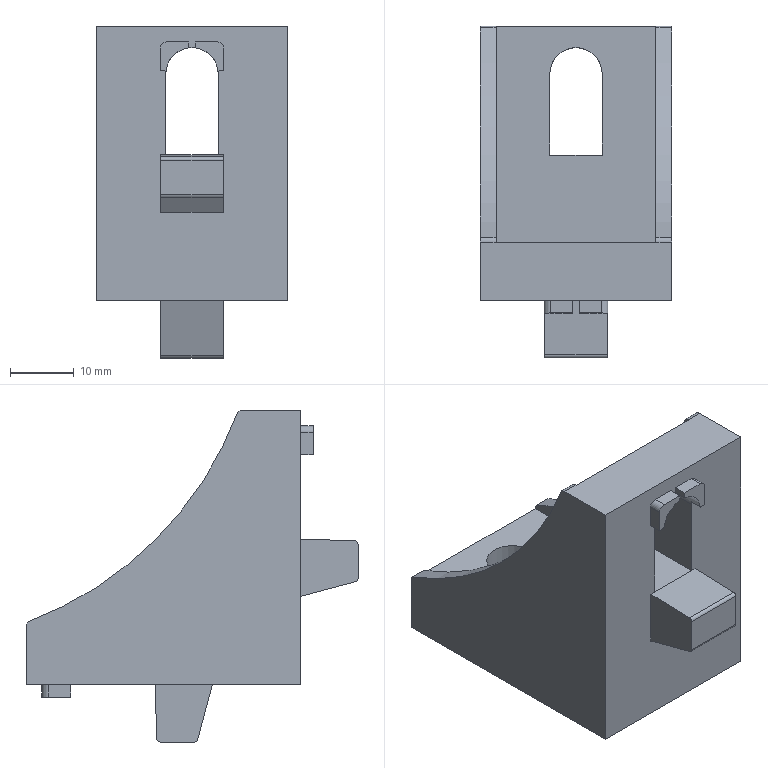Part | SolidWorks | features BaseBody 1 | 1 solid | 62 faces | box 30 x 52 x 52 mm | volume 22062 mm3 | plane 46 | cylinder 16 | commonest cylinder face diameters 2 x8 1 x4 8.2 x2 113.335 x2